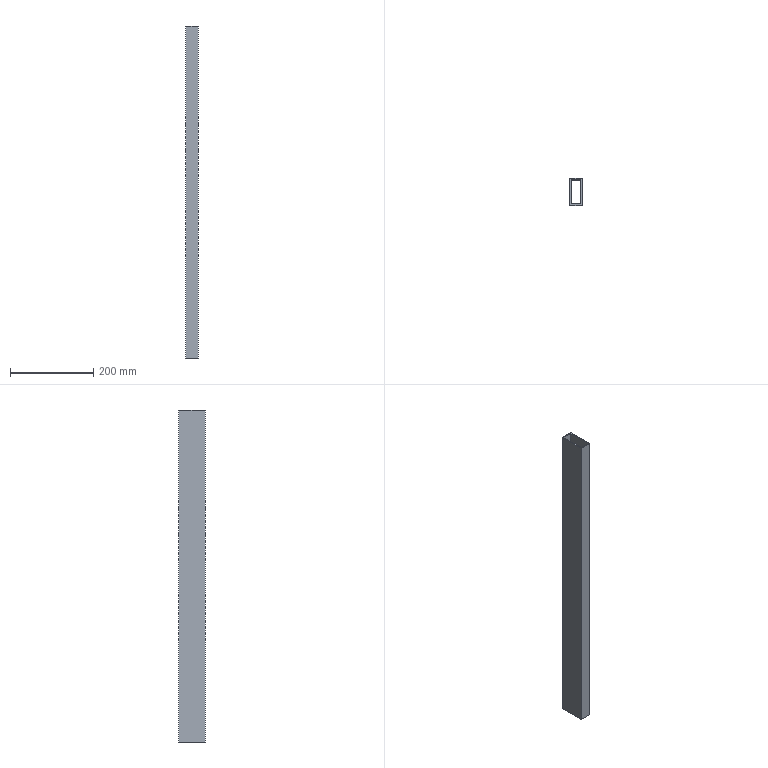Part | SolidWorks | features Extrusion 1, ICE 1 | 1 solid | 10 faces | box 30 x 65 x 800 mm | volume 427200 mm3 | plane 10
STEP:
#1=CARTESIAN_POINT('',(-10.853,38.973,0.));
#2=VERTEX_POINT('',#1);
#3=CARTESIAN_POINT('',(-40.853,38.973,0.));
#4=VERTEX_POINT('',#3);
#5=CARTESIAN_POINT('',(-10.853,38.973,0.));
#6=DIRECTION('',(-1.,0.,0.));
#7=VECTOR('',#6,1000.);
#8=LINE('',#5,#7);
#9=EDGE_CURVE('',#2,#4,#8,.T.);
#10=ORIENTED_EDGE('',*,*,#9,.T.);
#11=CARTESIAN_POINT('',(-40.853,38.973,800.));
#12=VERTEX_POINT('',#11);
#13=CARTESIAN_POINT('',(-40.853,38.973,800.));
#14=DIRECTION('',(0.,0.,-1.));
#15=VECTOR('',#14,1000.);
#16=LINE('',#13,#15);
#17=EDGE_CURVE('',#12,#4,#16,.T.);
#18=ORIENTED_EDGE('',*,*,#17,.F.);
#19=CARTESIAN_POINT('',(-10.853,38.973,800.));
#20=VERTEX_POINT('',#19);
#21=CARTESIAN_POINT('',(-10.853,38.973,800.));
#22=DIRECTION('',(-1.,0.,0.));
#23=VECTOR('',#22,1000.);
#24=LINE('',#21,#23);
#25=EDGE_CURVE('',#20,#12,#24,.T.);
#26=ORIENTED_EDGE('',*,*,#25,.F.);
#27=CARTESIAN_POINT('',(-10.853,38.973,800.));
#28=DIRECTION('',(0.,0.,-1.));
#29=VECTOR('',#28,1000.);
#30=LINE('',#27,#29);
#31=EDGE_CURVE('',#20,#2,#30,.T.);
#32=ORIENTED_EDGE('',*,*,#31,.T.);
#33=EDGE_LOOP('',(#10,#18,#26,#32));
#34=FACE_OUTER_BOUND('',#33,.T.);
#35=CARTESIAN_POINT('',(-10.853,38.973,800.));
#36=DIRECTION('',(0.,-1.,0.));
#37=DIRECTION('',(0.,0.,-1.));
#38=AXIS2_PLACEMENT_3D('',#35,#36,#37);
#39=PLANE('',#38);
#40=ADVANCED_FACE('',(#34),#39,.F.);
#41=CARTESIAN_POINT('',(-40.853,-26.027,0.));
#42=VERTEX_POINT('',#41);
#43=CARTESIAN_POINT('',(-40.853,38.973,0.));
#44=DIRECTION('',(0.,-1.,0.));
#45=VECTOR('',#44,1000.);
#46=LINE('',#43,#45);
#47=EDGE_CURVE('',#4,#42,#46,.T.);
#48=ORIENTED_EDGE('',*,*,#47,.T.);
#49=CARTESIAN_POINT('',(-40.853,-26.027,800.));
#50=VERTEX_POINT('',#49);
#51=CARTESIAN_POINT('',(-40.853,-26.027,800.));
#52=DIRECTION('',(0.,0.,-1.));
#53=VECTOR('',#52,1000.);
#54=LINE('',#51,#53);
#55=EDGE_CURVE('',#50,#42,#54,.T.);
#56=ORIENTED_EDGE('',*,*,#55,.F.);
#57=CARTESIAN_POINT('',(-40.853,38.973,800.));
#58=DIRECTION('',(0.,-1.,0.));
#59=VECTOR('',#58,1000.);
#60=LINE('',#57,#59);
#61=EDGE_CURVE('',#12,#50,#60,.T.);
#62=ORIENTED_EDGE('',*,*,#61,.F.);
#63=ORIENTED_EDGE('',*,*,#17,.T.);
#64=EDGE_LOOP('',(#48,#56,#62,#63));
#65=FACE_OUTER_BOUND('',#64,.T.);
#66=CARTESIAN_POINT('',(-40.853,38.973,800.));
#67=DIRECTION('',(1.,0.,0.));
#68=DIRECTION('',(0.,1.,0.));
#69=AXIS2_PLACEMENT_3D('',#66,#67,#68);
#70=PLANE('',#69);
#71=ADVANCED_FACE('',(#65),#70,.F.);
#72=CARTESIAN_POINT('',(-10.853,-26.027,0.));
#73=VERTEX_POINT('',#72);
#74=CARTESIAN_POINT('',(-40.853,-26.027,0.));
#75=DIRECTION('',(1.,0.,0.));
#76=VECTOR('',#75,1000.);
#77=LINE('',#74,#76);
#78=EDGE_CURVE('',#42,#73,#77,.T.);
#79=ORIENTED_EDGE('',*,*,#78,.T.);
#80=CARTESIAN_POINT('',(-10.853,-26.027,800.));
#81=VERTEX_POINT('',#80);
#82=CARTESIAN_POINT('',(-10.853,-26.027,800.));
#83=DIRECTION('',(0.,0.,-1.));
#84=VECTOR('',#83,1000.);
#85=LINE('',#82,#84);
#86=EDGE_CURVE('',#81,#73,#85,.T.);
#87=ORIENTED_EDGE('',*,*,#86,.F.);
#88=CARTESIAN_POINT('',(-40.853,-26.027,800.));
#89=DIRECTION('',(1.,0.,0.));
#90=VECTOR('',#89,1000.);
#91=LINE('',#88,#90);
#92=EDGE_CURVE('',#50,#81,#91,.T.);
#93=ORIENTED_EDGE('',*,*,#92,.F.);
#94=ORIENTED_EDGE('',*,*,#55,.T.);
#95=EDGE_LOOP('',(#79,#87,#93,#94));
#96=FACE_OUTER_BOUND('',#95,.T.);
#97=CARTESIAN_POINT('',(-40.853,-26.027,800.));
#98=DIRECTION('',(0.,1.,0.));
#99=DIRECTION('',(0.,0.,1.));
#100=AXIS2_PLACEMENT_3D('',#97,#98,#99);
#101=PLANE('',#100);
#102=ADVANCED_FACE('',(#96),#101,.F.);
#103=CARTESIAN_POINT('',(-10.853,-26.027,0.));
#104=DIRECTION('',(0.,1.,0.));
#105=VECTOR('',#104,1000.);
#106=LINE('',#103,#105);
#107=EDGE_CURVE('',#73,#2,#106,.T.);
#108=ORIENTED_EDGE('',*,*,#107,.T.);
#109=ORIENTED_EDGE('',*,*,#31,.F.);
#110=CARTESIAN_POINT('',(-10.853,-26.027,800.));
#111=DIRECTION('',(0.,1.,0.));
#112=VECTOR('',#111,1000.);
#113=LINE('',#110,#112);
#114=EDGE_CURVE('',#81,#20,#113,.T.);
#115=ORIENTED_EDGE('',*,*,#114,.F.);
#116=ORIENTED_EDGE('',*,*,#86,.T.);
#117=EDGE_LOOP('',(#108,#109,#115,#116));
#118=FACE_OUTER_BOUND('',#117,.T.);
#119=CARTESIAN_POINT('',(-10.853,-26.027,800.));
#120=DIRECTION('',(-1.,0.,0.));
#121=DIRECTION('',(0.,0.,1.));
#122=AXIS2_PLACEMENT_3D('',#119,#120,#121);
#123=PLANE('',#122);
#124=ADVANCED_FACE('',(#118),#123,.F.);
#125=CARTESIAN_POINT('',(-13.853,35.973,800.));
#126=VERTEX_POINT('',#125);
#127=CARTESIAN_POINT('',(-37.853,35.973,800.));
#128=VERTEX_POINT('',#127);
#129=CARTESIAN_POINT('',(-13.853,35.973,800.));
#130=DIRECTION('',(-1.,0.,0.));
#131=VECTOR('',#130,1000.);
#132=LINE('',#129,#131);
#133=EDGE_CURVE('',#126,#128,#132,.T.);
#134=ORIENTED_EDGE('',*,*,#133,.F.);
#135=CARTESIAN_POINT('',(-13.853,-23.027,800.));
#136=VERTEX_POINT('',#135);
#137=CARTESIAN_POINT('',(-13.853,-23.027,800.));
#138=DIRECTION('',(0.,1.,0.));
#139=VECTOR('',#138,1000.);
#140=LINE('',#137,#139);
#141=EDGE_CURVE('',#136,#126,#140,.T.);
#142=ORIENTED_EDGE('',*,*,#141,.F.);
#143=CARTESIAN_POINT('',(-37.853,-23.027,800.));
#144=VERTEX_POINT('',#143);
#145=CARTESIAN_POINT('',(-37.853,-23.027,800.));
#146=DIRECTION('',(1.,0.,0.));
#147=VECTOR('',#146,1000.);
#148=LINE('',#145,#147);
#149=EDGE_CURVE('',#144,#136,#148,.T.);
#150=ORIENTED_EDGE('',*,*,#149,.F.);
#151=CARTESIAN_POINT('',(-37.853,35.207,800.));
#152=DIRECTION('',(0.,-1.,0.));
#153=VECTOR('',#152,1000.);
#154=LINE('',#151,#153);
#155=EDGE_CURVE('',#128,#144,#154,.T.);
#156=ORIENTED_EDGE('',*,*,#155,.F.);
#157=EDGE_LOOP('',(#134,#142,#150,#156));
#158=FACE_BOUND('',#157,.T.);
#159=ORIENTED_EDGE('',*,*,#25,.T.);
#160=ORIENTED_EDGE('',*,*,#61,.T.);
#161=ORIENTED_EDGE('',*,*,#92,.T.);
#162=ORIENTED_EDGE('',*,*,#114,.T.);
#163=EDGE_LOOP('',(#159,#160,#161,#162));
#164=FACE_OUTER_BOUND('',#163,.T.);
#165=CARTESIAN_POINT('',(0.,0.,800.));
#166=DIRECTION('',(0.,0.,1.));
#167=DIRECTION('',(1.,0.,0.));
#168=AXIS2_PLACEMENT_3D('',#165,#166,#167);
#169=PLANE('',#168);
#170=ADVANCED_FACE('',(#158,#164),#169,.T.);
#171=CARTESIAN_POINT('',(-13.853,-23.027,0.));
#172=VERTEX_POINT('',#171);
#173=CARTESIAN_POINT('',(-13.853,35.973,0.));
#174=VERTEX_POINT('',#173);
#175=CARTESIAN_POINT('',(-13.853,-23.027,0.));
#176=DIRECTION('',(0.,1.,0.));
#177=VECTOR('',#176,1000.);
#178=LINE('',#175,#177);
#179=EDGE_CURVE('',#172,#174,#178,.T.);
#180=ORIENTED_EDGE('',*,*,#179,.T.);
#181=CARTESIAN_POINT('',(-37.853,35.973,0.));
#182=VERTEX_POINT('',#181);
#183=CARTESIAN_POINT('',(-13.853,35.973,0.));
#184=DIRECTION('',(-1.,0.,0.));
#185=VECTOR('',#184,1000.);
#186=LINE('',#183,#185);
#187=EDGE_CURVE('',#174,#182,#186,.T.);
#188=ORIENTED_EDGE('',*,*,#187,.T.);
#189=CARTESIAN_POINT('',(-37.853,-23.027,0.));
#190=VERTEX_POINT('',#189);
#191=CARTESIAN_POINT('',(-37.853,35.207,0.));
#192=DIRECTION('',(0.,-1.,0.));
#193=VECTOR('',#192,1000.);
#194=LINE('',#191,#193);
#195=EDGE_CURVE('',#182,#190,#194,.T.);
#196=ORIENTED_EDGE('',*,*,#195,.T.);
#197=CARTESIAN_POINT('',(-37.853,-23.027,0.));
#198=DIRECTION('',(1.,0.,0.));
#199=VECTOR('',#198,1000.);
#200=LINE('',#197,#199);
#201=EDGE_CURVE('',#190,#172,#200,.T.);
#202=ORIENTED_EDGE('',*,*,#201,.T.);
#203=EDGE_LOOP('',(#180,#188,#196,#202));
#204=FACE_BOUND('',#203,.T.);
#205=ORIENTED_EDGE('',*,*,#9,.F.);
#206=ORIENTED_EDGE('',*,*,#107,.F.);
#207=ORIENTED_EDGE('',*,*,#78,.F.);
#208=ORIENTED_EDGE('',*,*,#47,.F.);
#209=EDGE_LOOP('',(#205,#206,#207,#208));
#210=FACE_OUTER_BOUND('',#209,.T.);
#211=CARTESIAN_POINT('',(0.,0.,0.));
#212=DIRECTION('',(0.,0.,1.));
#213=DIRECTION('',(1.,0.,0.));
#214=AXIS2_PLACEMENT_3D('',#211,#212,#213);
#215=PLANE('',#214);
#216=ADVANCED_FACE('',(#204,#210),#215,.F.);
#217=ORIENTED_EDGE('',*,*,#133,.T.);
#218=CARTESIAN_POINT('',(-37.853,35.973,0.));
#219=DIRECTION('',(0.,0.,1.));
#220=VECTOR('',#219,1000.);
#221=LINE('',#218,#220);
#222=EDGE_CURVE('',#182,#128,#221,.T.);
#223=ORIENTED_EDGE('',*,*,#222,.F.);
#224=ORIENTED_EDGE('',*,*,#187,.F.);
#225=CARTESIAN_POINT('',(-13.853,35.973,0.));
#226=DIRECTION('',(0.,0.,1.));
#227=VECTOR('',#226,1000.);
#228=LINE('',#225,#227);
#229=EDGE_CURVE('',#174,#126,#228,.T.);
#230=ORIENTED_EDGE('',*,*,#229,.T.);
#231=EDGE_LOOP('',(#217,#223,#224,#230));
#232=FACE_OUTER_BOUND('',#231,.T.);
#233=CARTESIAN_POINT('',(-13.853,35.973,0.));
#234=DIRECTION('',(0.,1.,0.));
#235=DIRECTION('',(0.,0.,1.));
#236=AXIS2_PLACEMENT_3D('',#233,#234,#235);
#237=PLANE('',#236);
#238=ADVANCED_FACE('',(#232),#237,.F.);
#239=ORIENTED_EDGE('',*,*,#141,.T.);
#240=ORIENTED_EDGE('',*,*,#229,.F.);
#241=ORIENTED_EDGE('',*,*,#179,.F.);
#242=CARTESIAN_POINT('',(-13.853,-23.027,0.));
#243=DIRECTION('',(0.,0.,1.));
#244=VECTOR('',#243,1000.);
#245=LINE('',#242,#244);
#246=EDGE_CURVE('',#172,#136,#245,.T.);
#247=ORIENTED_EDGE('',*,*,#246,.T.);
#248=EDGE_LOOP('',(#239,#240,#241,#247));
#249=FACE_OUTER_BOUND('',#248,.T.);
#250=CARTESIAN_POINT('',(-13.853,-23.027,0.));
#251=DIRECTION('',(1.,0.,0.));
#252=DIRECTION('',(0.,0.,-1.));
#253=AXIS2_PLACEMENT_3D('',#250,#251,#252);
#254=PLANE('',#253);
#255=ADVANCED_FACE('',(#249),#254,.F.);
#256=ORIENTED_EDGE('',*,*,#149,.T.);
#257=ORIENTED_EDGE('',*,*,#246,.F.);
#258=ORIENTED_EDGE('',*,*,#201,.F.);
#259=CARTESIAN_POINT('',(-37.853,-23.027,0.));
#260=DIRECTION('',(0.,0.,1.));
#261=VECTOR('',#260,1000.);
#262=LINE('',#259,#261);
#263=EDGE_CURVE('',#190,#144,#262,.T.);
#264=ORIENTED_EDGE('',*,*,#263,.T.);
#265=EDGE_LOOP('',(#256,#257,#258,#264));
#266=FACE_OUTER_BOUND('',#265,.T.);
#267=CARTESIAN_POINT('',(-37.853,-23.027,0.));
#268=DIRECTION('',(0.,-1.,0.));
#269=DIRECTION('',(0.,0.,-1.));
#270=AXIS2_PLACEMENT_3D('',#267,#268,#269);
#271=PLANE('',#270);
#272=ADVANCED_FACE('',(#266),#271,.F.);
#273=ORIENTED_EDGE('',*,*,#155,.T.);
#274=ORIENTED_EDGE('',*,*,#263,.F.);
#275=ORIENTED_EDGE('',*,*,#195,.F.);
#276=ORIENTED_EDGE('',*,*,#222,.T.);
#277=EDGE_LOOP('',(#273,#274,#275,#276));
#278=FACE_OUTER_BOUND('',#277,.T.);
#279=CARTESIAN_POINT('',(-37.853,35.207,0.));
#280=DIRECTION('',(-1.,0.,0.));
#281=DIRECTION('',(0.,-1.,0.));
#282=AXIS2_PLACEMENT_3D('',#279,#280,#281);
#283=PLANE('',#282);
#284=ADVANCED_FACE('',(#278),#283,.F.);
#285=CLOSED_SHELL('',(#40,#71,#102,#124,#170,#216,#238,#255,#272,#284));
#286=MANIFOLD_SOLID_BREP('',#285);
#287=CARTESIAN_POINT('',(0.,0.,0.));
#288=DIRECTION('',(0.,0.,1.));
#289=DIRECTION('',(1.,0.,0.));
#290=AXIS2_PLACEMENT_3D('',#287,#288,#289);
#291=(LENGTH_UNIT()NAMED_UNIT(*)SI_UNIT(.MILLI.,.METRE.));
#292=UNCERTAINTY_MEASURE_WITH_UNIT(LENGTH_MEASURE(0.00001),#291,'','');
#293=(NAMED_UNIT(*)PLANE_ANGLE_UNIT()SI_UNIT($,.RADIAN.));
#294=(NAMED_UNIT(*)SI_UNIT($,.STERADIAN.)SOLID_ANGLE_UNIT());
#295=(GEOMETRIC_REPRESENTATION_CONTEXT(3)GLOBAL_UNCERTAINTY_ASSIGNED_CONTEXT((#292))GLOBAL_UNIT_ASSIGNED_CONTEXT((#291,#293,#294))REPRESENTATION_CONTEXT('',''));
#296=ADVANCED_BREP_SHAPE_REPRESENTATION('',(#286,#290),#295);